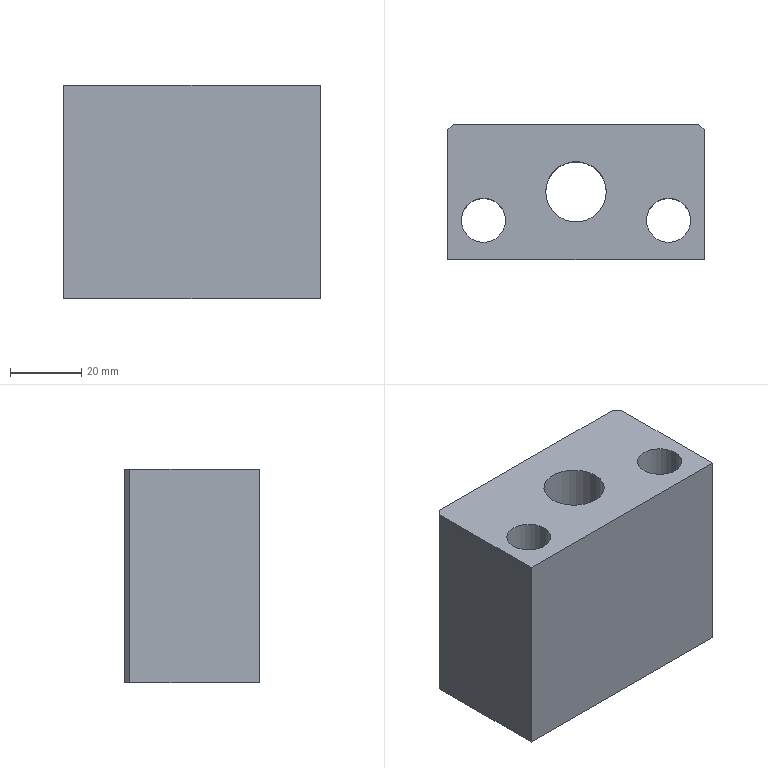Part | STEP file | Mount electronic clip rodless cylinder 2-2-2 | 1 solid | 38 faces | box 72 x 38 x 60 mm | volume 135352 mm3 | cone 16 | cylinder 14 | plane 8 | commonest cylinder face diameters 4.13 x8 12.4 x4 17 x2